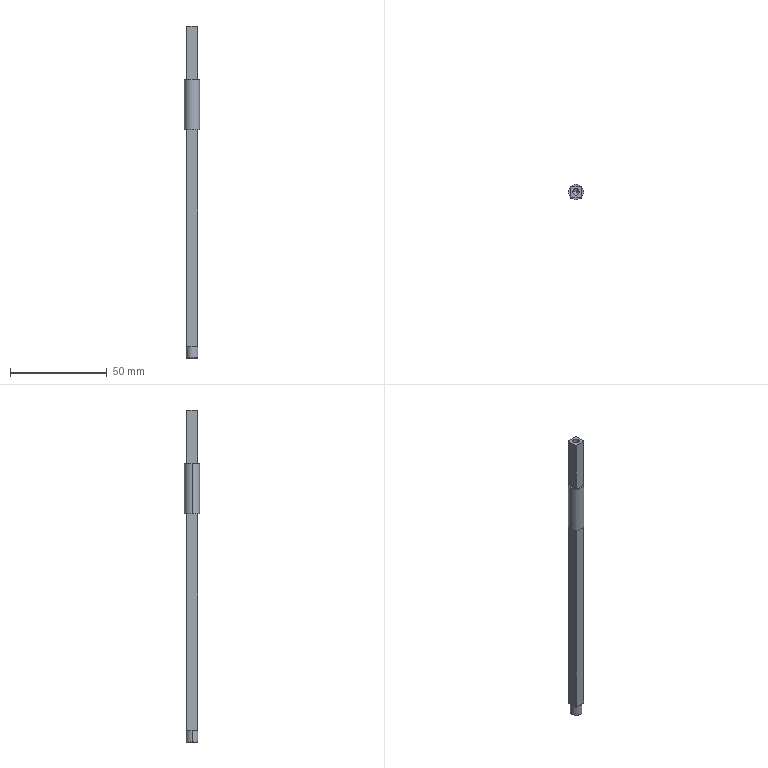Part | NX | features BREP 1 | 1 solid | 36 faces | box 8 x 8 x 172 mm | volume 6270 mm3 | plane 22 | cylinder 8 | cone 6 | commonest cylinder face diameters 3.3 x4 6 x2 8 x2
STEP:
#1=CARTESIAN_POINT('',(-3.,0.,-88.85));
#2=VERTEX_POINT('',#1);
#3=CARTESIAN_POINT('',(-2.85,0.,-89.));
#4=VERTEX_POINT('',#3);
#5=CARTESIAN_POINT('',(-3.,0.,-88.85));
#6=DIRECTION('',(-0.7071,0.,0.7071));
#7=VECTOR('',#6,1000.);
#8=LINE('',#5,#7);
#9=EDGE_CURVE('',#2,#4,#8,.F.);
#10=ORIENTED_EDGE('',*,*,#9,.T.);
#11=CARTESIAN_POINT('',(2.85,0.,-89.));
#12=VERTEX_POINT('',#11);
#13=CARTESIAN_POINT('',(0.,0.,-89.));
#14=DIRECTION('',(0.,0.,-1.));
#15=DIRECTION('',(1.,0.,0.));
#16=AXIS2_PLACEMENT_3D('',#13,#14,#15);
#17=CIRCLE('',#16,2.85);
#18=EDGE_CURVE('',#12,#4,#17,.T.);
#19=ORIENTED_EDGE('',*,*,#18,.F.);
#20=CARTESIAN_POINT('',(3.,0.,-88.85));
#21=VERTEX_POINT('',#20);
#22=CARTESIAN_POINT('',(3.,0.,-88.85));
#23=DIRECTION('',(0.7071,0.,0.7071));
#24=VECTOR('',#23,1000.);
#25=LINE('',#22,#24);
#26=EDGE_CURVE('',#21,#12,#25,.F.);
#27=ORIENTED_EDGE('',*,*,#26,.F.);
#28=CARTESIAN_POINT('',(0.,0.,-88.85));
#29=DIRECTION('',(0.,0.,1.));
#30=DIRECTION('',(1.,0.,0.));
#31=AXIS2_PLACEMENT_3D('',#28,#29,#30);
#32=CIRCLE('',#31,3.);
#33=EDGE_CURVE('',#2,#21,#32,.T.);
#34=ORIENTED_EDGE('',*,*,#33,.F.);
#35=EDGE_LOOP('',(#10,#19,#27,#34));
#36=FACE_BOUND('',#35,.T.);
#37=CARTESIAN_POINT('',(0.,0.,-88.85));
#38=DIRECTION('',(0.,0.,1.));
#39=DIRECTION('',(1.,0.,0.));
#40=AXIS2_PLACEMENT_3D('',#37,#38,#39);
#41=CONICAL_SURFACE('',#40,3.,0.7854);
#42=ADVANCED_FACE('',(#36),#41,.T.);
#43=CARTESIAN_POINT('',(1.65,0.,-76.9));
#44=VERTEX_POINT('',#43);
#45=CARTESIAN_POINT('',(1.65,0.,-89.));
#46=VERTEX_POINT('',#45);
#47=CARTESIAN_POINT('',(1.65,0.,-89.));
#48=DIRECTION('',(0.,0.,-1.));
#49=VECTOR('',#48,1000.);
#50=LINE('',#47,#49);
#51=EDGE_CURVE('',#44,#46,#50,.T.);
#52=ORIENTED_EDGE('',*,*,#51,.F.);
#53=CARTESIAN_POINT('',(-1.65,0.,-76.9));
#54=VERTEX_POINT('',#53);
#55=CARTESIAN_POINT('',(0.,0.,-76.9));
#56=DIRECTION('',(0.,0.,-1.));
#57=DIRECTION('',(-1.,0.,0.));
#58=AXIS2_PLACEMENT_3D('',#55,#56,#57);
#59=CIRCLE('',#58,1.65);
#60=EDGE_CURVE('',#54,#44,#59,.T.);
#61=ORIENTED_EDGE('',*,*,#60,.F.);
#62=CARTESIAN_POINT('',(-1.65,0.,-89.));
#63=VERTEX_POINT('',#62);
#64=CARTESIAN_POINT('',(-1.65,0.,-89.));
#65=DIRECTION('',(0.,0.,-1.));
#66=VECTOR('',#65,1000.);
#67=LINE('',#64,#66);
#68=EDGE_CURVE('',#54,#63,#67,.T.);
#69=ORIENTED_EDGE('',*,*,#68,.T.);
#70=CARTESIAN_POINT('',(0.,0.,-89.));
#71=DIRECTION('',(0.,0.,-1.));
#72=DIRECTION('',(-1.,0.,0.));
#73=AXIS2_PLACEMENT_3D('',#70,#71,#72);
#74=CIRCLE('',#73,1.65);
#75=EDGE_CURVE('',#63,#46,#74,.T.);
#76=ORIENTED_EDGE('',*,*,#75,.T.);
#77=EDGE_LOOP('',(#52,#61,#69,#76));
#78=FACE_BOUND('',#77,.T.);
#79=CARTESIAN_POINT('',(0.,0.,-89.));
#80=DIRECTION('',(0.,0.,-1.));
#81=DIRECTION('',(-1.,0.,0.));
#82=AXIS2_PLACEMENT_3D('',#79,#80,#81);
#83=CYLINDRICAL_SURFACE('',#82,1.65);
#84=ADVANCED_FACE('',(#78),#83,.F.);
#85=CARTESIAN_POINT('',(0.,0.,-75.909));
#86=VERTEX_POINT('',#85);
#87=CARTESIAN_POINT('',(1.65,0.,-76.9));
#88=DIRECTION('',(0.8572,0.,-0.515));
#89=VECTOR('',#88,1000.);
#90=LINE('',#87,#89);
#91=EDGE_CURVE('',#44,#86,#90,.F.);
#92=ORIENTED_EDGE('',*,*,#91,.T.);
#93=CARTESIAN_POINT('',(-1.65,0.,-76.9));
#94=DIRECTION('',(-0.8572,0.,-0.515));
#95=VECTOR('',#94,1000.);
#96=LINE('',#93,#95);
#97=EDGE_CURVE('',#54,#86,#96,.F.);
#98=ORIENTED_EDGE('',*,*,#97,.F.);
#99=ORIENTED_EDGE('',*,*,#60,.T.);
#100=EDGE_LOOP('',(#92,#98,#99));
#101=FACE_BOUND('',#100,.T.);
#102=CARTESIAN_POINT('',(0.,0.,-76.9));
#103=DIRECTION('',(0.,0.,-1.));
#104=DIRECTION('',(-1.,0.,0.));
#105=AXIS2_PLACEMENT_3D('',#102,#103,#104);
#106=CONICAL_SURFACE('',#105,1.65,1.03);
#107=ADVANCED_FACE('',(#101),#106,.F.);
#108=CARTESIAN_POINT('',(-1.65,0.,83.));
#109=VERTEX_POINT('',#108);
#110=CARTESIAN_POINT('',(-1.65,0.,70.9));
#111=VERTEX_POINT('',#110);
#112=CARTESIAN_POINT('',(-1.65,0.,83.));
#113=DIRECTION('',(0.,0.,1.));
#114=VECTOR('',#113,1000.);
#115=LINE('',#112,#114);
#116=EDGE_CURVE('',#109,#111,#115,.F.);
#117=ORIENTED_EDGE('',*,*,#116,.T.);
#118=CARTESIAN_POINT('',(1.65,0.,70.9));
#119=VERTEX_POINT('',#118);
#120=CARTESIAN_POINT('',(0.,0.,70.9));
#121=DIRECTION('',(0.,0.,1.));
#122=DIRECTION('',(1.,0.,0.));
#123=AXIS2_PLACEMENT_3D('',#120,#121,#122);
#124=CIRCLE('',#123,1.65);
#125=EDGE_CURVE('',#119,#111,#124,.T.);
#126=ORIENTED_EDGE('',*,*,#125,.F.);
#127=CARTESIAN_POINT('',(1.65,0.,83.));
#128=VERTEX_POINT('',#127);
#129=CARTESIAN_POINT('',(1.65,0.,83.));
#130=DIRECTION('',(0.,0.,1.));
#131=VECTOR('',#130,1000.);
#132=LINE('',#129,#131);
#133=EDGE_CURVE('',#128,#119,#132,.F.);
#134=ORIENTED_EDGE('',*,*,#133,.F.);
#135=CARTESIAN_POINT('',(0.,0.,83.));
#136=DIRECTION('',(0.,0.,1.));
#137=DIRECTION('',(1.,0.,0.));
#138=AXIS2_PLACEMENT_3D('',#135,#136,#137);
#139=CIRCLE('',#138,1.65);
#140=EDGE_CURVE('',#128,#109,#139,.T.);
#141=ORIENTED_EDGE('',*,*,#140,.T.);
#142=EDGE_LOOP('',(#117,#126,#134,#141));
#143=FACE_BOUND('',#142,.T.);
#144=CARTESIAN_POINT('',(0.,0.,83.));
#145=DIRECTION('',(0.,0.,1.));
#146=DIRECTION('',(1.,0.,0.));
#147=AXIS2_PLACEMENT_3D('',#144,#145,#146);
#148=CYLINDRICAL_SURFACE('',#147,1.65);
#149=ADVANCED_FACE('',(#143),#148,.F.);
#150=CARTESIAN_POINT('',(0.,0.,69.909));
#151=VERTEX_POINT('',#150);
#152=CARTESIAN_POINT('',(-1.65,0.,70.9));
#153=DIRECTION('',(-0.8572,0.,0.515));
#154=VECTOR('',#153,1000.);
#155=LINE('',#152,#154);
#156=EDGE_CURVE('',#151,#111,#155,.T.);
#157=ORIENTED_EDGE('',*,*,#156,.F.);
#158=CARTESIAN_POINT('',(1.65,0.,70.9));
#159=DIRECTION('',(0.8572,0.,0.515));
#160=VECTOR('',#159,1000.);
#161=LINE('',#158,#160);
#162=EDGE_CURVE('',#151,#119,#161,.T.);
#163=ORIENTED_EDGE('',*,*,#162,.T.);
#164=ORIENTED_EDGE('',*,*,#125,.T.);
#165=EDGE_LOOP('',(#157,#163,#164));
#166=FACE_BOUND('',#165,.T.);
#167=CARTESIAN_POINT('',(0.,0.,70.9));
#168=DIRECTION('',(0.,0.,1.));
#169=DIRECTION('',(1.,0.,0.));
#170=AXIS2_PLACEMENT_3D('',#167,#168,#169);
#171=CONICAL_SURFACE('',#170,1.65,1.03);
#172=ADVANCED_FACE('',(#166),#171,.F.);
#173=CARTESIAN_POINT('',(-2.646,-3.,55.25));
#174=VERTEX_POINT('',#173);
#175=CARTESIAN_POINT('',(2.646,-3.,55.25));
#176=VERTEX_POINT('',#175);
#177=CARTESIAN_POINT('',(-2.646,-3.,55.25));
#178=DIRECTION('',(1.,0.,0.));
#179=VECTOR('',#178,1000.);
#180=LINE('',#177,#179);
#181=EDGE_CURVE('',#174,#176,#180,.T.);
#182=ORIENTED_EDGE('',*,*,#181,.F.);
#183=CARTESIAN_POINT('',(0.,0.,55.25));
#184=DIRECTION('',(0.,0.,1.));
#185=DIRECTION('',(1.,0.,0.));
#186=AXIS2_PLACEMENT_3D('',#183,#184,#185);
#187=CIRCLE('',#186,4.);
#188=EDGE_CURVE('',#174,#176,#187,.T.);
#189=ORIENTED_EDGE('',*,*,#188,.T.);
#190=EDGE_LOOP('',(#182,#189));
#191=FACE_BOUND('',#190,.T.);
#192=CARTESIAN_POINT('',(0.,0.,55.25));
#193=DIRECTION('',(0.,0.,1.));
#194=DIRECTION('',(1.,0.,0.));
#195=AXIS2_PLACEMENT_3D('',#192,#193,#194);
#196=PLANE('',#195);
#197=ADVANCED_FACE('',(#191),#196,.T.);
#198=CARTESIAN_POINT('',(-2.646,-3.,29.25));
#199=VERTEX_POINT('',#198);
#200=CARTESIAN_POINT('',(2.646,-3.,29.25));
#201=VERTEX_POINT('',#200);
#202=CARTESIAN_POINT('',(0.,0.,29.25));
#203=DIRECTION('',(0.,0.,1.));
#204=DIRECTION('',(1.,0.,0.));
#205=AXIS2_PLACEMENT_3D('',#202,#203,#204);
#206=CIRCLE('',#205,4.);
#207=EDGE_CURVE('',#199,#201,#206,.T.);
#208=ORIENTED_EDGE('',*,*,#207,.F.);
#209=CARTESIAN_POINT('',(-2.646,-3.,29.25));
#210=DIRECTION('',(1.,0.,0.));
#211=VECTOR('',#210,1000.);
#212=LINE('',#209,#211);
#213=EDGE_CURVE('',#199,#201,#212,.T.);
#214=ORIENTED_EDGE('',*,*,#213,.T.);
#215=EDGE_LOOP('',(#208,#214));
#216=FACE_BOUND('',#215,.T.);
#217=CARTESIAN_POINT('',(0.,0.,29.25));
#218=DIRECTION('',(0.,0.,1.));
#219=DIRECTION('',(1.,0.,0.));
#220=AXIS2_PLACEMENT_3D('',#217,#218,#219);
#221=PLANE('',#220);
#222=ADVANCED_FACE('',(#216),#221,.F.);
#223=CARTESIAN_POINT('',(3.,-2.646,29.25));
#224=VERTEX_POINT('',#223);
#225=CARTESIAN_POINT('',(4.,0.,29.25));
#226=VERTEX_POINT('',#225);
#227=CARTESIAN_POINT('',(0.,0.,29.25));
#228=DIRECTION('',(0.,0.,1.));
#229=DIRECTION('',(1.,0.,0.));
#230=AXIS2_PLACEMENT_3D('',#227,#228,#229);
#231=CIRCLE('',#230,4.);
#232=EDGE_CURVE('',#224,#226,#231,.T.);
#233=ORIENTED_EDGE('',*,*,#232,.F.);
#234=CARTESIAN_POINT('',(3.,2.646,29.25));
#235=VERTEX_POINT('',#234);
#236=CARTESIAN_POINT('',(3.,-2.646,29.25));
#237=DIRECTION('',(0.,1.,0.));
#238=VECTOR('',#237,1000.);
#239=LINE('',#236,#238);
#240=EDGE_CURVE('',#224,#235,#239,.T.);
#241=ORIENTED_EDGE('',*,*,#240,.T.);
#242=CARTESIAN_POINT('',(0.,0.,29.25));
#243=DIRECTION('',(0.,0.,1.));
#244=DIRECTION('',(1.,0.,0.));
#245=AXIS2_PLACEMENT_3D('',#242,#243,#244);
#246=CIRCLE('',#245,4.);
#247=EDGE_CURVE('',#226,#235,#246,.T.);
#248=ORIENTED_EDGE('',*,*,#247,.F.);
#249=EDGE_LOOP('',(#233,#241,#248));
#250=FACE_BOUND('',#249,.T.);
#251=CARTESIAN_POINT('',(0.,0.,29.25));
#252=DIRECTION('',(0.,0.,1.));
#253=DIRECTION('',(1.,0.,0.));
#254=AXIS2_PLACEMENT_3D('',#251,#252,#253);
#255=PLANE('',#254);
#256=ADVANCED_FACE('',(#250),#255,.F.);
#257=CARTESIAN_POINT('',(3.,-2.646,55.25));
#258=VERTEX_POINT('',#257);
#259=CARTESIAN_POINT('',(3.,2.646,55.25));
#260=VERTEX_POINT('',#259);
#261=CARTESIAN_POINT('',(3.,-2.646,55.25));
#262=DIRECTION('',(0.,1.,0.));
#263=VECTOR('',#262,1000.);
#264=LINE('',#261,#263);
#265=EDGE_CURVE('',#258,#260,#264,.T.);
#266=ORIENTED_EDGE('',*,*,#265,.F.);
#267=CARTESIAN_POINT('',(4.,0.,55.25));
#268=VERTEX_POINT('',#267);
#269=CARTESIAN_POINT('',(0.,0.,55.25));
#270=DIRECTION('',(0.,0.,1.));
#271=DIRECTION('',(1.,0.,0.));
#272=AXIS2_PLACEMENT_3D('',#269,#270,#271);
#273=CIRCLE('',#272,4.);
#274=EDGE_CURVE('',#258,#268,#273,.T.);
#275=ORIENTED_EDGE('',*,*,#274,.T.);
#276=CARTESIAN_POINT('',(0.,0.,55.25));
#277=DIRECTION('',(0.,0.,1.));
#278=DIRECTION('',(1.,0.,0.));
#279=AXIS2_PLACEMENT_3D('',#276,#277,#278);
#280=CIRCLE('',#279,4.);
#281=EDGE_CURVE('',#268,#260,#280,.T.);
#282=ORIENTED_EDGE('',*,*,#281,.T.);
#283=EDGE_LOOP('',(#266,#275,#282));
#284=FACE_BOUND('',#283,.T.);
#285=CARTESIAN_POINT('',(0.,0.,55.25));
#286=DIRECTION('',(0.,0.,1.));
#287=DIRECTION('',(1.,0.,0.));
#288=AXIS2_PLACEMENT_3D('',#285,#286,#287);
#289=PLANE('',#288);
#290=ADVANCED_FACE('',(#284),#289,.T.);
#291=CARTESIAN_POINT('',(2.646,3.,29.25));
#292=VERTEX_POINT('',#291);
#293=CARTESIAN_POINT('',(-2.646,3.,29.25));
#294=VERTEX_POINT('',#293);
#295=CARTESIAN_POINT('',(0.,0.,29.25));
#296=DIRECTION('',(0.,0.,1.));
#297=DIRECTION('',(1.,0.,0.));
#298=AXIS2_PLACEMENT_3D('',#295,#296,#297);
#299=CIRCLE('',#298,4.);
#300=EDGE_CURVE('',#292,#294,#299,.T.);
#301=ORIENTED_EDGE('',*,*,#300,.F.);
#302=CARTESIAN_POINT('',(-2.646,3.,29.25));
#303=DIRECTION('',(-1.,0.,0.));
#304=VECTOR('',#303,1000.);
#305=LINE('',#302,#304);
#306=EDGE_CURVE('',#292,#294,#305,.T.);
#307=ORIENTED_EDGE('',*,*,#306,.T.);
#308=EDGE_LOOP('',(#301,#307));
#309=FACE_BOUND('',#308,.T.);
#310=CARTESIAN_POINT('',(0.,0.,29.25));
#311=DIRECTION('',(0.,0.,1.));
#312=DIRECTION('',(1.,0.,0.));
#313=AXIS2_PLACEMENT_3D('',#310,#311,#312);
#314=PLANE('',#313);
#315=ADVANCED_FACE('',(#309),#314,.F.);
#316=CARTESIAN_POINT('',(2.646,3.,55.25));
#317=VERTEX_POINT('',#316);
#318=CARTESIAN_POINT('',(-2.646,3.,55.25));
#319=VERTEX_POINT('',#318);
#320=CARTESIAN_POINT('',(-2.646,3.,55.25));
#321=DIRECTION('',(-1.,0.,0.));
#322=VECTOR('',#321,1000.);
#323=LINE('',#320,#322);
#324=EDGE_CURVE('',#317,#319,#323,.T.);
#325=ORIENTED_EDGE('',*,*,#324,.F.);
#326=CARTESIAN_POINT('',(0.,0.,55.25));
#327=DIRECTION('',(0.,0.,1.));
#328=DIRECTION('',(1.,0.,0.));
#329=AXIS2_PLACEMENT_3D('',#326,#327,#328);
#330=CIRCLE('',#329,4.);
#331=EDGE_CURVE('',#317,#319,#330,.T.);
#332=ORIENTED_EDGE('',*,*,#331,.T.);
#333=EDGE_LOOP('',(#325,#332));
#334=FACE_BOUND('',#333,.T.);
#335=CARTESIAN_POINT('',(0.,0.,55.25));
#336=DIRECTION('',(0.,0.,1.));
#337=DIRECTION('',(1.,0.,0.));
#338=AXIS2_PLACEMENT_3D('',#335,#336,#337);
#339=PLANE('',#338);
#340=ADVANCED_FACE('',(#334),#339,.T.);
#341=CARTESIAN_POINT('',(-3.,2.646,29.25));
#342=VERTEX_POINT('',#341);
#343=CARTESIAN_POINT('',(-4.,0.,29.25));
#344=VERTEX_POINT('',#343);
#345=CARTESIAN_POINT('',(0.,0.,29.25));
#346=DIRECTION('',(0.,0.,1.));
#347=DIRECTION('',(1.,0.,0.));
#348=AXIS2_PLACEMENT_3D('',#345,#346,#347);
#349=CIRCLE('',#348,4.);
#350=EDGE_CURVE('',#342,#344,#349,.T.);
#351=ORIENTED_EDGE('',*,*,#350,.F.);
#352=CARTESIAN_POINT('',(-3.,-2.646,29.25));
#353=VERTEX_POINT('',#352);
#354=CARTESIAN_POINT('',(-3.,-2.646,29.25));
#355=DIRECTION('',(0.,-1.,0.));
#356=VECTOR('',#355,1000.);
#357=LINE('',#354,#356);
#358=EDGE_CURVE('',#342,#353,#357,.T.);
#359=ORIENTED_EDGE('',*,*,#358,.T.);
#360=CARTESIAN_POINT('',(0.,0.,29.25));
#361=DIRECTION('',(0.,0.,1.));
#362=DIRECTION('',(1.,0.,0.));
#363=AXIS2_PLACEMENT_3D('',#360,#361,#362);
#364=CIRCLE('',#363,4.);
#365=EDGE_CURVE('',#344,#353,#364,.T.);
#366=ORIENTED_EDGE('',*,*,#365,.F.);
#367=EDGE_LOOP('',(#351,#359,#366));
#368=FACE_BOUND('',#367,.T.);
#369=CARTESIAN_POINT('',(0.,0.,29.25));
#370=DIRECTION('',(0.,0.,1.));
#371=DIRECTION('',(1.,0.,0.));
#372=AXIS2_PLACEMENT_3D('',#369,#370,#371);
#373=PLANE('',#372);
#374=ADVANCED_FACE('',(#368),#373,.F.);
#375=CARTESIAN_POINT('',(-3.,2.646,55.25));
#376=VERTEX_POINT('',#375);
#377=CARTESIAN_POINT('',(-3.,-2.646,55.25));
#378=VERTEX_POINT('',#377);
#379=CARTESIAN_POINT('',(-3.,-2.646,55.25));
#380=DIRECTION('',(0.,-1.,0.));
#381=VECTOR('',#380,1000.);
#382=LINE('',#379,#381);
#383=EDGE_CURVE('',#376,#378,#382,.T.);
#384=ORIENTED_EDGE('',*,*,#383,.F.);
#385=CARTESIAN_POINT('',(-4.,0.,55.25));
#386=VERTEX_POINT('',#385);
#387=CARTESIAN_POINT('',(0.,0.,55.25));
#388=DIRECTION('',(0.,0.,1.));
#389=DIRECTION('',(1.,0.,0.));
#390=AXIS2_PLACEMENT_3D('',#387,#388,#389);
#391=CIRCLE('',#390,4.);
#392=EDGE_CURVE('',#376,#386,#391,.T.);
#393=ORIENTED_EDGE('',*,*,#392,.T.);
#394=CARTESIAN_POINT('',(0.,0.,55.25));
#395=DIRECTION('',(0.,0.,1.));
#396=DIRECTION('',(1.,0.,0.));
#397=AXIS2_PLACEMENT_3D('',#394,#395,#396);
#398=CIRCLE('',#397,4.);
#399=EDGE_CURVE('',#386,#378,#398,.T.);
#400=ORIENTED_EDGE('',*,*,#399,.T.);
#401=EDGE_LOOP('',(#384,#393,#400));
#402=FACE_BOUND('',#401,.T.);
#403=CARTESIAN_POINT('',(0.,0.,55.25));
#404=DIRECTION('',(0.,0.,1.));
#405=DIRECTION('',(1.,0.,0.));
#406=AXIS2_PLACEMENT_3D('',#403,#404,#405);
#407=PLANE('',#406);
#408=ADVANCED_FACE('',(#402),#407,.T.);
#409=ORIENTED_EDGE('',*,*,#75,.F.);
#410=CARTESIAN_POINT('',(0.,0.,-89.));
#411=DIRECTION('',(0.,0.,-1.));
#412=DIRECTION('',(-1.,0.,0.));
#413=AXIS2_PLACEMENT_3D('',#410,#411,#412);
#414=CIRCLE('',#413,1.65);
#415=EDGE_CURVE('',#46,#63,#414,.T.);
#416=ORIENTED_EDGE('',*,*,#415,.F.);
#417=EDGE_LOOP('',(#409,#416));
#418=FACE_BOUND('',#417,.T.);
#419=ORIENTED_EDGE('',*,*,#18,.T.);
#420=CARTESIAN_POINT('',(0.,0.,-89.));
#421=DIRECTION('',(0.,0.,-1.));
#422=DIRECTION('',(1.,0.,0.));
#423=AXIS2_PLACEMENT_3D('',#420,#421,#422);
#424=CIRCLE('',#423,2.85);
#425=EDGE_CURVE('',#4,#12,#424,.T.);
#426=ORIENTED_EDGE('',*,*,#425,.T.);
#427=EDGE_LOOP('',(#419,#426));
#428=FACE_BOUND('',#427,.T.);
#429=CARTESIAN_POINT('',(-3.,0.,-89.));
#430=DIRECTION('',(0.,0.,1.));
#431=DIRECTION('',(1.,0.,0.));
#432=AXIS2_PLACEMENT_3D('',#429,#430,#431);
#433=PLANE('',#432);
#434=ADVANCED_FACE('',(#418,#428),#433,.F.);
#435=CARTESIAN_POINT('',(-3.,0.,-83.));
#436=VERTEX_POINT('',#435);
#437=CARTESIAN_POINT('',(-3.,0.,0.));
#438=DIRECTION('',(0.,0.,1.));
#439=VECTOR('',#438,1000.);
#440=LINE('',#437,#439);
#441=EDGE_CURVE('',#436,#2,#440,.F.);
#442=ORIENTED_EDGE('',*,*,#441,.T.);
#443=ORIENTED_EDGE('',*,*,#33,.T.);
#444=CARTESIAN_POINT('',(3.,0.,-83.));
#445=VERTEX_POINT('',#444);
#446=CARTESIAN_POINT('',(3.,0.,0.));
#447=DIRECTION('',(0.,0.,1.));
#448=VECTOR('',#447,1000.);
#449=LINE('',#446,#448);
#450=EDGE_CURVE('',#445,#21,#449,.F.);
#451=ORIENTED_EDGE('',*,*,#450,.F.);
#452=CARTESIAN_POINT('',(0.,-3.,-83.));
#453=VERTEX_POINT('',#452);
#454=CARTESIAN_POINT('',(0.,0.,-83.));
#455=DIRECTION('',(0.,0.,1.));
#456=DIRECTION('',(1.,0.,0.));
#457=AXIS2_PLACEMENT_3D('',#454,#455,#456);
#458=CIRCLE('',#457,3.);
#459=EDGE_CURVE('',#453,#445,#458,.T.);
#460=ORIENTED_EDGE('',*,*,#459,.F.);
#461=CARTESIAN_POINT('',(0.,0.,-83.));
#462=DIRECTION('',(0.,0.,1.));
#463=DIRECTION('',(1.,0.,0.));
#464=AXIS2_PLACEMENT_3D('',#461,#462,#463);
#465=CIRCLE('',#464,3.);
#466=EDGE_CURVE('',#436,#453,#465,.T.);
#467=ORIENTED_EDGE('',*,*,#466,.F.);
#468=EDGE_LOOP('',(#442,#443,#451,#460,#467));
#469=FACE_BOUND('',#468,.T.);
#470=CARTESIAN_POINT('',(0.,0.,0.));
#471=DIRECTION('',(0.,0.,1.));
#472=DIRECTION('',(1.,0.,0.));
#473=AXIS2_PLACEMENT_3D('',#470,#471,#472);
#474=CYLINDRICAL_SURFACE('',#473,3.);
#475=ADVANCED_FACE('',(#469),#474,.T.);
#476=CARTESIAN_POINT('',(2.646,-3.,-83.));
#477=VERTEX_POINT('',#476);
#478=CARTESIAN_POINT('',(-2.646,-3.,-83.));
#479=DIRECTION('',(1.,0.,0.));
#480=VECTOR('',#479,1000.);
#481=LINE('',#478,#480);
#482=EDGE_CURVE('',#453,#477,#481,.T.);
#483=ORIENTED_EDGE('',*,*,#482,.F.);
#484=ORIENTED_EDGE('',*,*,#459,.T.);
#485=CARTESIAN_POINT('',(3.,-2.646,-83.));
#486=VERTEX_POINT('',#485);
#487=CARTESIAN_POINT('',(3.,-2.646,-83.));
#488=DIRECTION('',(0.,1.,0.));
#489=VECTOR('',#488,1000.);
#490=LINE('',#487,#489);
#491=EDGE_CURVE('',#486,#445,#490,.T.);
#492=ORIENTED_EDGE('',*,*,#491,.F.);
#493=CARTESIAN_POINT('',(0.,0.,-83.));
#494=DIRECTION('',(0.,0.,1.));
#495=DIRECTION('',(1.,0.,0.));
#496=AXIS2_PLACEMENT_3D('',#493,#494,#495);
#497=CIRCLE('',#496,4.);
#498=EDGE_CURVE('',#477,#486,#497,.T.);
#499=ORIENTED_EDGE('',*,*,#498,.F.);
#500=EDGE_LOOP('',(#483,#484,#492,#499));
#501=FACE_BOUND('',#500,.T.);
#502=CARTESIAN_POINT('',(0.,0.,-83.));
#503=DIRECTION('',(0.,0.,1.));
#504=DIRECTION('',(1.,0.,0.));
#505=AXIS2_PLACEMENT_3D('',#502,#503,#504);
#506=PLANE('',#505);
#507=ADVANCED_FACE('',(#501),#506,.F.);
#508=CARTESIAN_POINT('',(-3.,-2.646,83.));
#509=VERTEX_POINT('',#508);
#510=CARTESIAN_POINT('',(-2.646,-3.,83.));
#511=VERTEX_POINT('',#510);
#512=CARTESIAN_POINT('',(0.,0.,83.));
#513=DIRECTION('',(0.,0.,1.));
#514=DIRECTION('',(1.,0.,0.));
#515=AXIS2_PLACEMENT_3D('',#512,#513,#514);
#516=CIRCLE('',#515,4.);
#517=EDGE_CURVE('',#509,#511,#516,.T.);
#518=ORIENTED_EDGE('',*,*,#517,.T.);
#519=CARTESIAN_POINT('',(2.646,-3.,83.));
#520=VERTEX_POINT('',#519);
#521=CARTESIAN_POINT('',(-2.646,-3.,83.));
#522=DIRECTION('',(1.,0.,0.));
#523=VECTOR('',#522,1000.);
#524=LINE('',#521,#523);
#525=EDGE_CURVE('',#511,#520,#524,.T.);
#526=ORIENTED_EDGE('',*,*,#525,.T.);
#527=CARTESIAN_POINT('',(3.,-2.646,83.));
#528=VERTEX_POINT('',#527);
#529=CARTESIAN_POINT('',(0.,0.,83.));
#530=DIRECTION('',(0.,0.,1.));
#531=DIRECTION('',(1.,0.,0.));
#532=AXIS2_PLACEMENT_3D('',#529,#530,#531);
#533=CIRCLE('',#532,4.);
#534=EDGE_CURVE('',#520,#528,#533,.T.);
#535=ORIENTED_EDGE('',*,*,#534,.T.);
#536=CARTESIAN_POINT('',(3.,2.646,83.));
#537=VERTEX_POINT('',#536);
#538=CARTESIAN_POINT('',(3.,-2.646,83.));
#539=DIRECTION('',(0.,1.,0.));
#540=VECTOR('',#539,1000.);
#541=LINE('',#538,#540);
#542=EDGE_CURVE('',#528,#537,#541,.T.);
#543=ORIENTED_EDGE('',*,*,#542,.T.);
#544=CARTESIAN_POINT('',(2.646,3.,83.));
#545=VERTEX_POINT('',#544);
#546=CARTESIAN_POINT('',(0.,0.,83.));
#547=DIRECTION('',(0.,0.,1.));
#548=DIRECTION('',(1.,0.,0.));
#549=AXIS2_PLACEMENT_3D('',#546,#547,#548);
#550=CIRCLE('',#549,4.);
#551=EDGE_CURVE('',#537,#545,#550,.T.);
#552=ORIENTED_EDGE('',*,*,#551,.T.);
#553=CARTESIAN_POINT('',(-2.646,3.,83.));
#554=VERTEX_POINT('',#553);
#555=CARTESIAN_POINT('',(-2.646,3.,83.));
#556=DIRECTION('',(-1.,0.,0.));
#557=VECTOR('',#556,1000.);
#558=LINE('',#555,#557);
#559=EDGE_CURVE('',#545,#554,#558,.T.);
#560=ORIENTED_EDGE('',*,*,#559,.T.);
#561=CARTESIAN_POINT('',(-3.,2.646,83.));
#562=VERTEX_POINT('',#561);
#563=CARTESIAN_POINT('',(0.,0.,83.));
#564=DIRECTION('',(0.,0.,1.));
#565=DIRECTION('',(1.,0.,0.));
#566=AXIS2_PLACEMENT_3D('',#563,#564,#565);
#567=CIRCLE('',#566,4.);
#568=EDGE_CURVE('',#554,#562,#567,.T.);
#569=ORIENTED_EDGE('',*,*,#568,.T.);
#570=CARTESIAN_POINT('',(-3.,-2.646,83.));
#571=DIRECTION('',(0.,-1.,0.));
#572=VECTOR('',#571,1000.);
#573=LINE('',#570,#572);
#574=EDGE_CURVE('',#562,#509,#573,.T.);
#575=ORIENTED_EDGE('',*,*,#574,.T.);
#576=EDGE_LOOP('',(#518,#526,#535,#543,#552,#560,#569,#575));
#577=FACE_BOUND('',#576,.T.);
#578=ORIENTED_EDGE('',*,*,#140,.F.);
#579=CARTESIAN_POINT('',(0.,0.,83.));
#580=DIRECTION('',(0.,0.,1.));
#581=DIRECTION('',(1.,0.,0.));
#582=AXIS2_PLACEMENT_3D('',#579,#580,#581);
#583=CIRCLE('',#582,1.65);
#584=EDGE_CURVE('',#109,#128,#583,.T.);
#585=ORIENTED_EDGE('',*,*,#584,.F.);
#586=EDGE_LOOP('',(#578,#585));
#587=FACE_BOUND('',#586,.T.);
#588=CARTESIAN_POINT('',(0.,0.,83.));
#589=DIRECTION('',(0.,0.,1.));
#590=DIRECTION('',(1.,0.,0.));
#591=AXIS2_PLACEMENT_3D('',#588,#589,#590);
#592=PLANE('',#591);
#593=ADVANCED_FACE('',(#577,#587),#592,.T.);
#594=CARTESIAN_POINT('',(-3.,2.646,83.));
#595=DIRECTION('',(0.,0.,-1.));
#596=VECTOR('',#595,1000.);
#597=LINE('',#594,#596);
#598=EDGE_CURVE('',#562,#376,#597,.T.);
#599=ORIENTED_EDGE('',*,*,#598,.T.);
#600=ORIENTED_EDGE('',*,*,#383,.T.);
#601=CARTESIAN_POINT('',(-3.,-2.646,83.));
#602=DIRECTION('',(0.,0.,-1.));
#603=VECTOR('',#602,1000.);
#604=LINE('',#601,#603);
#605=EDGE_CURVE('',#509,#378,#604,.T.);
#606=ORIENTED_EDGE('',*,*,#605,.F.);
#607=ORIENTED_EDGE('',*,*,#574,.F.);
#608=EDGE_LOOP('',(#599,#600,#606,#607));
#609=FACE_BOUND('',#608,.T.);
#610=CARTESIAN_POINT('',(-3.,-2.646,83.));
#611=DIRECTION('',(1.,0.,0.));
#612=DIRECTION('',(0.,0.,-1.));
#613=AXIS2_PLACEMENT_3D('',#610,#611,#612);
#614=PLANE('',#613);
#615=ADVANCED_FACE('',(#609),#614,.F.);
#616=CARTESIAN_POINT('',(4.,0.,83.));
#617=DIRECTION('',(0.,0.,-1.));
#618=VECTOR('',#617,1000.);
#619=LINE('',#616,#618);
#620=EDGE_CURVE('',#268,#226,#619,.T.);
#621=ORIENTED_EDGE('',*,*,#620,.F.);
#622=ORIENTED_EDGE('',*,*,#274,.F.);
#623=CARTESIAN_POINT('',(3.,-2.646,83.));
#624=DIRECTION('',(0.,0.,-1.));
#625=VECTOR('',#624,1000.);
#626=LINE('',#623,#625);
#627=EDGE_CURVE('',#528,#258,#626,.T.);
#628=ORIENTED_EDGE('',*,*,#627,.F.);
#629=ORIENTED_EDGE('',*,*,#534,.F.);
#630=CARTESIAN_POINT('',(2.646,-3.,83.));
#631=DIRECTION('',(0.,0.,-1.));
#632=VECTOR('',#631,1000.);
#633=LINE('',#630,#632);
#634=EDGE_CURVE('',#176,#520,#633,.F.);
#635=ORIENTED_EDGE('',*,*,#634,.F.);
#636=ORIENTED_EDGE('',*,*,#188,.F.);
#637=CARTESIAN_POINT('',(-2.646,-3.,83.));
#638=DIRECTION('',(0.,0.,-1.));
#639=VECTOR('',#638,1000.);
#640=LINE('',#637,#639);
#641=EDGE_CURVE('',#174,#511,#640,.F.);
#642=ORIENTED_EDGE('',*,*,#641,.T.);
#643=ORIENTED_EDGE('',*,*,#517,.F.);
#644=ORIENTED_EDGE('',*,*,#605,.T.);
#645=ORIENTED_EDGE('',*,*,#399,.F.);
#646=CARTESIAN_POINT('',(-4.,0.,83.));
#647=DIRECTION('',(0.,0.,-1.));
#648=VECTOR('',#647,1000.);
#649=LINE('',#646,#648);
#650=EDGE_CURVE('',#386,#344,#649,.T.);
#651=ORIENTED_EDGE('',*,*,#650,.T.);
#652=ORIENTED_EDGE('',*,*,#365,.T.);
#653=CARTESIAN_POINT('',(-3.,-2.646,-83.));
#654=VERTEX_POINT('',#653);
#655=CARTESIAN_POINT('',(-3.,-2.646,83.));
#656=DIRECTION('',(0.,0.,-1.));
#657=VECTOR('',#656,1000.);
#658=LINE('',#655,#657);
#659=EDGE_CURVE('',#353,#654,#658,.T.);
#660=ORIENTED_EDGE('',*,*,#659,.T.);
#661=CARTESIAN_POINT('',(-2.646,-3.,-83.));
#662=VERTEX_POINT('',#661);
#663=CARTESIAN_POINT('',(0.,0.,-83.));
#664=DIRECTION('',(0.,0.,1.));
#665=DIRECTION('',(1.,0.,0.));
#666=AXIS2_PLACEMENT_3D('',#663,#664,#665);
#667=CIRCLE('',#666,4.);
#668=EDGE_CURVE('',#654,#662,#667,.T.);
#669=ORIENTED_EDGE('',*,*,#668,.T.);
#670=CARTESIAN_POINT('',(-2.646,-3.,83.));
#671=DIRECTION('',(0.,0.,-1.));
#672=VECTOR('',#671,1000.);
#673=LINE('',#670,#672);
#674=EDGE_CURVE('',#662,#199,#673,.F.);
#675=ORIENTED_EDGE('',*,*,#674,.T.);
#676=ORIENTED_EDGE('',*,*,#207,.T.);
#677=CARTESIAN_POINT('',(2.646,-3.,83.));
#678=DIRECTION('',(0.,0.,-1.));
#679=VECTOR('',#678,1000.);
#680=LINE('',#677,#679);
#681=EDGE_CURVE('',#477,#201,#680,.F.);
#682=ORIENTED_EDGE('',*,*,#681,.F.);
#683=ORIENTED_EDGE('',*,*,#498,.T.);
#684=CARTESIAN_POINT('',(3.,-2.646,83.));
#685=DIRECTION('',(0.,0.,-1.));
#686=VECTOR('',#685,1000.);
#687=LINE('',#684,#686);
#688=EDGE_CURVE('',#224,#486,#687,.T.);
#689=ORIENTED_EDGE('',*,*,#688,.F.);
#690=ORIENTED_EDGE('',*,*,#232,.T.);
#691=EDGE_LOOP('',(#621,#622,#628,#629,#635,#636,#642,#643,#644,#645,#651,#652,#660,#669,#675,#676,#682,#683,#689,#690));
#692=FACE_BOUND('',#691,.T.);
#693=CARTESIAN_POINT('',(0.,0.,83.));
#694=DIRECTION('',(0.,0.,-1.));
#695=DIRECTION('',(-1.,0.,0.));
#696=AXIS2_PLACEMENT_3D('',#693,#694,#695);
#697=CYLINDRICAL_SURFACE('',#696,4.);
#698=ADVANCED_FACE('',(#692),#697,.T.);
#699=CARTESIAN_POINT('',(2.646,3.,83.));
#700=DIRECTION('',(0.,0.,-1.));
#701=VECTOR('',#700,1000.);
#702=LINE('',#699,#701);
#703=EDGE_CURVE('',#317,#545,#702,.F.);
#704=ORIENTED_EDGE('',*,*,#703,.F.);
#705=ORIENTED_EDGE('',*,*,#324,.T.);
#706=CARTESIAN_POINT('',(-2.646,3.,83.));
#707=DIRECTION('',(0.,0.,-1.));
#708=VECTOR('',#707,1000.);
#709=LINE('',#706,#708);
#710=EDGE_CURVE('',#319,#554,#709,.F.);
#711=ORIENTED_EDGE('',*,*,#710,.T.);
#712=ORIENTED_EDGE('',*,*,#559,.F.);
#713=EDGE_LOOP('',(#704,#705,#711,#712));
#714=FACE_BOUND('',#713,.T.);
#715=CARTESIAN_POINT('',(-2.646,3.,83.));
#716=DIRECTION('',(0.,-1.,0.));
#717=DIRECTION('',(0.,0.,-1.));
#718=AXIS2_PLACEMENT_3D('',#715,#716,#717);
#719=PLANE('',#718);
#720=ADVANCED_FACE('',(#714),#719,.F.);
#721=ORIENTED_EDGE('',*,*,#627,.T.);
#722=ORIENTED_EDGE('',*,*,#265,.T.);
#723=CARTESIAN_POINT('',(3.,2.646,83.));
#724=DIRECTION('',(0.,0.,-1.));
#725=VECTOR('',#724,1000.);
#726=LINE('',#723,#725);
#727=EDGE_CURVE('',#537,#260,#726,.T.);
#728=ORIENTED_EDGE('',*,*,#727,.F.);
#729=ORIENTED_EDGE('',*,*,#542,.F.);
#730=EDGE_LOOP('',(#721,#722,#728,#729));
#731=FACE_BOUND('',#730,.T.);
#732=CARTESIAN_POINT('',(3.,-2.646,83.));
#733=DIRECTION('',(-1.,0.,0.));
#734=DIRECTION('',(0.,-1.,0.));
#735=AXIS2_PLACEMENT_3D('',#732,#733,#734);
#736=PLANE('',#735);
#737=ADVANCED_FACE('',(#731),#736,.F.);
#738=ORIENTED_EDGE('',*,*,#641,.F.);
#739=ORIENTED_EDGE('',*,*,#181,.T.);
#740=ORIENTED_EDGE('',*,*,#634,.T.);
#741=ORIENTED_EDGE('',*,*,#525,.F.);
#742=EDGE_LOOP('',(#738,#739,#740,#741));
#743=FACE_BOUND('',#742,.T.);
#744=CARTESIAN_POINT('',(-2.646,-3.,83.));
#745=DIRECTION('',(0.,1.,0.));
#746=DIRECTION('',(0.,0.,1.));
#747=AXIS2_PLACEMENT_3D('',#744,#745,#746);
#748=PLANE('',#747);
#749=ADVANCED_FACE('',(#743),#748,.F.);
#750=CARTESIAN_POINT('',(-3.,-2.646,-83.));
#751=DIRECTION('',(0.,-1.,0.));
#752=VECTOR('',#751,1000.);
#753=LINE('',#750,#752);
#754=EDGE_CURVE('',#436,#654,#753,.T.);
#755=ORIENTED_EDGE('',*,*,#754,.F.);
#756=ORIENTED_EDGE('',*,*,#466,.T.);
#757=CARTESIAN_POINT('',(-2.646,-3.,-83.));
#758=DIRECTION('',(1.,0.,0.));
#759=VECTOR('',#758,1000.);
#760=LINE('',#757,#759);
#761=EDGE_CURVE('',#662,#453,#760,.T.);
#762=ORIENTED_EDGE('',*,*,#761,.F.);
#763=ORIENTED_EDGE('',*,*,#668,.F.);
#764=EDGE_LOOP('',(#755,#756,#762,#763));
#765=FACE_BOUND('',#764,.T.);
#766=CARTESIAN_POINT('',(0.,0.,-83.));
#767=DIRECTION('',(0.,0.,1.));
#768=DIRECTION('',(1.,0.,0.));
#769=AXIS2_PLACEMENT_3D('',#766,#767,#768);
#770=PLANE('',#769);
#771=ADVANCED_FACE('',(#765),#770,.F.);
#772=CARTESIAN_POINT('',(0.,3.,-83.));
#773=VERTEX_POINT('',#772);
#774=CARTESIAN_POINT('',(-2.646,3.,-83.));
#775=VERTEX_POINT('',#774);
#776=CARTESIAN_POINT('',(-2.646,3.,-83.));
#777=DIRECTION('',(-1.,0.,0.));
#778=VECTOR('',#777,1000.);
#779=LINE('',#776,#778);
#780=EDGE_CURVE('',#773,#775,#779,.T.);
#781=ORIENTED_EDGE('',*,*,#780,.F.);
#782=CARTESIAN_POINT('',(0.,0.,-83.));
#783=DIRECTION('',(0.,0.,1.));
#784=DIRECTION('',(1.,0.,0.));
#785=AXIS2_PLACEMENT_3D('',#782,#783,#784);
#786=CIRCLE('',#785,3.);
#787=EDGE_CURVE('',#773,#436,#786,.T.);
#788=ORIENTED_EDGE('',*,*,#787,.T.);
#789=CARTESIAN_POINT('',(-3.,2.646,-83.));
#790=VERTEX_POINT('',#789);
#791=CARTESIAN_POINT('',(-3.,-2.646,-83.));
#792=DIRECTION('',(0.,-1.,0.));
#793=VECTOR('',#792,1000.);
#794=LINE('',#791,#793);
#795=EDGE_CURVE('',#790,#436,#794,.T.);
#796=ORIENTED_EDGE('',*,*,#795,.F.);
#797=CARTESIAN_POINT('',(0.,0.,-83.));
#798=DIRECTION('',(0.,0.,1.));
#799=DIRECTION('',(1.,0.,0.));
#800=AXIS2_PLACEMENT_3D('',#797,#798,#799);
#801=CIRCLE('',#800,4.);
#802=EDGE_CURVE('',#775,#790,#801,.T.);
#803=ORIENTED_EDGE('',*,*,#802,.F.);
#804=EDGE_LOOP('',(#781,#788,#796,#803));
#805=FACE_BOUND('',#804,.T.);
#806=CARTESIAN_POINT('',(0.,0.,-83.));
#807=DIRECTION('',(0.,0.,1.));
#808=DIRECTION('',(1.,0.,0.));
#809=AXIS2_PLACEMENT_3D('',#806,#807,#808);
#810=PLANE('',#809);
#811=ADVANCED_FACE('',(#805),#810,.F.);
#812=CARTESIAN_POINT('',(3.,2.646,-83.));
#813=VERTEX_POINT('',#812);
#814=CARTESIAN_POINT('',(3.,-2.646,-83.));
#815=DIRECTION('',(0.,1.,0.));
#816=VECTOR('',#815,1000.);
#817=LINE('',#814,#816);
#818=EDGE_CURVE('',#445,#813,#817,.T.);
#819=ORIENTED_EDGE('',*,*,#818,.F.);
#820=CARTESIAN_POINT('',(0.,0.,-83.));
#821=DIRECTION('',(0.,0.,1.));
#822=DIRECTION('',(1.,0.,0.));
#823=AXIS2_PLACEMENT_3D('',#820,#821,#822);
#824=CIRCLE('',#823,3.);
#825=EDGE_CURVE('',#445,#773,#824,.T.);
#826=ORIENTED_EDGE('',*,*,#825,.T.);
#827=CARTESIAN_POINT('',(2.646,3.,-83.));
#828=VERTEX_POINT('',#827);
#829=CARTESIAN_POINT('',(-2.646,3.,-83.));
#830=DIRECTION('',(-1.,0.,0.));
#831=VECTOR('',#830,1000.);
#832=LINE('',#829,#831);
#833=EDGE_CURVE('',#828,#773,#832,.T.);
#834=ORIENTED_EDGE('',*,*,#833,.F.);
#835=CARTESIAN_POINT('',(0.,0.,-83.));
#836=DIRECTION('',(0.,0.,1.));
#837=DIRECTION('',(1.,0.,0.));
#838=AXIS2_PLACEMENT_3D('',#835,#836,#837);
#839=CIRCLE('',#838,4.);
#840=EDGE_CURVE('',#813,#828,#839,.T.);
#841=ORIENTED_EDGE('',*,*,#840,.F.);
#842=EDGE_LOOP('',(#819,#826,#834,#841));
#843=FACE_BOUND('',#842,.T.);
#844=CARTESIAN_POINT('',(0.,0.,-83.));
#845=DIRECTION('',(0.,0.,1.));
#846=DIRECTION('',(1.,0.,0.));
#847=AXIS2_PLACEMENT_3D('',#844,#845,#846);
#848=PLANE('',#847);
#849=ADVANCED_FACE('',(#843),#848,.F.);
#850=ORIENTED_EDGE('',*,*,#358,.F.);
#851=CARTESIAN_POINT('',(-3.,2.646,83.));
#852=DIRECTION('',(0.,0.,-1.));
#853=VECTOR('',#852,1000.);
#854=LINE('',#851,#853);
#855=EDGE_CURVE('',#342,#790,#854,.T.);
#856=ORIENTED_EDGE('',*,*,#855,.T.);
#857=ORIENTED_EDGE('',*,*,#795,.T.);
#858=ORIENTED_EDGE('',*,*,#754,.T.);
#859=ORIENTED_EDGE('',*,*,#659,.F.);
#860=EDGE_LOOP('',(#850,#856,#857,#858,#859));
#861=FACE_BOUND('',#860,.T.);
#862=CARTESIAN_POINT('',(-3.,-2.646,83.));
#863=DIRECTION('',(1.,0.,0.));
#864=DIRECTION('',(0.,0.,-1.));
#865=AXIS2_PLACEMENT_3D('',#862,#863,#864);
#866=PLANE('',#865);
#867=ADVANCED_FACE('',(#861),#866,.F.);
#868=ORIENTED_EDGE('',*,*,#306,.F.);
#869=CARTESIAN_POINT('',(2.646,3.,83.));
#870=DIRECTION('',(0.,0.,-1.));
#871=VECTOR('',#870,1000.);
#872=LINE('',#869,#871);
#873=EDGE_CURVE('',#292,#828,#872,.T.);
#874=ORIENTED_EDGE('',*,*,#873,.T.);
#875=ORIENTED_EDGE('',*,*,#833,.T.);
#876=ORIENTED_EDGE('',*,*,#780,.T.);
#877=CARTESIAN_POINT('',(-2.646,3.,83.));
#878=DIRECTION('',(0.,0.,-1.));
#879=VECTOR('',#878,1000.);
#880=LINE('',#877,#879);
#881=EDGE_CURVE('',#294,#775,#880,.T.);
#882=ORIENTED_EDGE('',*,*,#881,.F.);
#883=EDGE_LOOP('',(#868,#874,#875,#876,#882));
#884=FACE_BOUND('',#883,.T.);
#885=CARTESIAN_POINT('',(-2.646,3.,83.));
#886=DIRECTION('',(0.,-1.,0.));
#887=DIRECTION('',(0.,0.,-1.));
#888=AXIS2_PLACEMENT_3D('',#885,#886,#887);
#889=PLANE('',#888);
#890=ADVANCED_FACE('',(#884),#889,.F.);
#891=ORIENTED_EDGE('',*,*,#240,.F.);
#892=ORIENTED_EDGE('',*,*,#688,.T.);
#893=ORIENTED_EDGE('',*,*,#491,.T.);
#894=ORIENTED_EDGE('',*,*,#818,.T.);
#895=CARTESIAN_POINT('',(3.,2.646,83.));
#896=DIRECTION('',(0.,0.,-1.));
#897=VECTOR('',#896,1000.);
#898=LINE('',#895,#897);
#899=EDGE_CURVE('',#235,#813,#898,.T.);
#900=ORIENTED_EDGE('',*,*,#899,.F.);
#901=EDGE_LOOP('',(#891,#892,#893,#894,#900));
#902=FACE_BOUND('',#901,.T.);
#903=CARTESIAN_POINT('',(3.,-2.646,83.));
#904=DIRECTION('',(-1.,0.,0.));
#905=DIRECTION('',(0.,-1.,0.));
#906=AXIS2_PLACEMENT_3D('',#903,#904,#905);
#907=PLANE('',#906);
#908=ADVANCED_FACE('',(#902),#907,.F.);
#909=ORIENTED_EDGE('',*,*,#213,.F.);
#910=ORIENTED_EDGE('',*,*,#674,.F.);
#911=ORIENTED_EDGE('',*,*,#761,.T.);
#912=ORIENTED_EDGE('',*,*,#482,.T.);
#913=ORIENTED_EDGE('',*,*,#681,.T.);
#914=EDGE_LOOP('',(#909,#910,#911,#912,#913));
#915=FACE_BOUND('',#914,.T.);
#916=CARTESIAN_POINT('',(-2.646,-3.,83.));
#917=DIRECTION('',(0.,1.,0.));
#918=DIRECTION('',(0.,0.,1.));
#919=AXIS2_PLACEMENT_3D('',#916,#917,#918);
#920=PLANE('',#919);
#921=ADVANCED_FACE('',(#915),#920,.F.);
#922=ORIENTED_EDGE('',*,*,#281,.F.);
#923=ORIENTED_EDGE('',*,*,#620,.T.);
#924=ORIENTED_EDGE('',*,*,#247,.T.);
#925=ORIENTED_EDGE('',*,*,#899,.T.);
#926=ORIENTED_EDGE('',*,*,#840,.T.);
#927=ORIENTED_EDGE('',*,*,#873,.F.);
#928=ORIENTED_EDGE('',*,*,#300,.T.);
#929=ORIENTED_EDGE('',*,*,#881,.T.);
#930=ORIENTED_EDGE('',*,*,#802,.T.);
#931=ORIENTED_EDGE('',*,*,#855,.F.);
#932=ORIENTED_EDGE('',*,*,#350,.T.);
#933=ORIENTED_EDGE('',*,*,#650,.F.);
#934=ORIENTED_EDGE('',*,*,#392,.F.);
#935=ORIENTED_EDGE('',*,*,#598,.F.);
#936=ORIENTED_EDGE('',*,*,#568,.F.);
#937=ORIENTED_EDGE('',*,*,#710,.F.);
#938=ORIENTED_EDGE('',*,*,#331,.F.);
#939=ORIENTED_EDGE('',*,*,#703,.T.);
#940=ORIENTED_EDGE('',*,*,#551,.F.);
#941=ORIENTED_EDGE('',*,*,#727,.T.);
#942=EDGE_LOOP('',(#922,#923,#924,#925,#926,#927,#928,#929,#930,#931,#932,#933,#934,#935,#936,#937,#938,#939,#940,#941));
#943=FACE_BOUND('',#942,.T.);
#944=CARTESIAN_POINT('',(0.,0.,83.));
#945=DIRECTION('',(0.,0.,-1.));
#946=DIRECTION('',(-1.,0.,0.));
#947=AXIS2_PLACEMENT_3D('',#944,#945,#946);
#948=CYLINDRICAL_SURFACE('',#947,4.);
#949=ADVANCED_FACE('',(#943),#948,.T.);
#950=CARTESIAN_POINT('',(0.,0.,-88.85));
#951=DIRECTION('',(0.,0.,1.));
#952=DIRECTION('',(1.,0.,0.));
#953=AXIS2_PLACEMENT_3D('',#950,#951,#952);
#954=CIRCLE('',#953,3.);
#955=EDGE_CURVE('',#21,#2,#954,.T.);
#956=ORIENTED_EDGE('',*,*,#955,.T.);
#957=ORIENTED_EDGE('',*,*,#441,.F.);
#958=ORIENTED_EDGE('',*,*,#787,.F.);
#959=ORIENTED_EDGE('',*,*,#825,.F.);
#960=ORIENTED_EDGE('',*,*,#450,.T.);
#961=EDGE_LOOP('',(#956,#957,#958,#959,#960));
#962=FACE_BOUND('',#961,.T.);
#963=CARTESIAN_POINT('',(0.,0.,0.));
#964=DIRECTION('',(0.,0.,1.));
#965=DIRECTION('',(1.,0.,0.));
#966=AXIS2_PLACEMENT_3D('',#963,#964,#965);
#967=CYLINDRICAL_SURFACE('',#966,3.);
#968=ADVANCED_FACE('',(#962),#967,.T.);
#969=ORIENTED_EDGE('',*,*,#162,.F.);
#970=ORIENTED_EDGE('',*,*,#156,.T.);
#971=CARTESIAN_POINT('',(0.,0.,70.9));
#972=DIRECTION('',(0.,0.,1.));
#973=DIRECTION('',(1.,0.,0.));
#974=AXIS2_PLACEMENT_3D('',#971,#972,#973);
#975=CIRCLE('',#974,1.65);
#976=EDGE_CURVE('',#111,#119,#975,.T.);
#977=ORIENTED_EDGE('',*,*,#976,.T.);
#978=EDGE_LOOP('',(#969,#970,#977));
#979=FACE_BOUND('',#978,.T.);
#980=CARTESIAN_POINT('',(0.,0.,70.9));
#981=DIRECTION('',(0.,0.,1.));
#982=DIRECTION('',(1.,0.,0.));
#983=AXIS2_PLACEMENT_3D('',#980,#981,#982);
#984=CONICAL_SURFACE('',#983,1.65,1.03);
#985=ADVANCED_FACE('',(#979),#984,.F.);
#986=ORIENTED_EDGE('',*,*,#976,.F.);
#987=ORIENTED_EDGE('',*,*,#116,.F.);
#988=ORIENTED_EDGE('',*,*,#584,.T.);
#989=ORIENTED_EDGE('',*,*,#133,.T.);
#990=EDGE_LOOP('',(#986,#987,#988,#989));
#991=FACE_BOUND('',#990,.T.);
#992=CARTESIAN_POINT('',(0.,0.,83.));
#993=DIRECTION('',(0.,0.,1.));
#994=DIRECTION('',(1.,0.,0.));
#995=AXIS2_PLACEMENT_3D('',#992,#993,#994);
#996=CYLINDRICAL_SURFACE('',#995,1.65);
#997=ADVANCED_FACE('',(#991),#996,.F.);
#998=ORIENTED_EDGE('',*,*,#97,.T.);
#999=ORIENTED_EDGE('',*,*,#91,.F.);
#1000=CARTESIAN_POINT('',(0.,0.,-76.9));
#1001=DIRECTION('',(0.,0.,-1.));
#1002=DIRECTION('',(-1.,0.,0.));
#1003=AXIS2_PLACEMENT_3D('',#1000,#1001,#1002);
#1004=CIRCLE('',#1003,1.65);
#1005=EDGE_CURVE('',#44,#54,#1004,.T.);
#1006=ORIENTED_EDGE('',*,*,#1005,.T.);
#1007=EDGE_LOOP('',(#998,#999,#1006));
#1008=FACE_BOUND('',#1007,.T.);
#1009=CARTESIAN_POINT('',(0.,0.,-76.9));
#1010=DIRECTION('',(0.,0.,-1.));
#1011=DIRECTION('',(-1.,0.,0.));
#1012=AXIS2_PLACEMENT_3D('',#1009,#1010,#1011);
#1013=CONICAL_SURFACE('',#1012,1.65,1.03);
#1014=ADVANCED_FACE('',(#1008),#1013,.F.);
#1015=ORIENTED_EDGE('',*,*,#1005,.F.);
#1016=ORIENTED_EDGE('',*,*,#51,.T.);
#1017=ORIENTED_EDGE('',*,*,#415,.T.);
#1018=ORIENTED_EDGE('',*,*,#68,.F.);
#1019=EDGE_LOOP('',(#1015,#1016,#1017,#1018));
#1020=FACE_BOUND('',#1019,.T.);
#1021=CARTESIAN_POINT('',(0.,0.,-89.));
#1022=DIRECTION('',(0.,0.,-1.));
#1023=DIRECTION('',(-1.,0.,0.));
#1024=AXIS2_PLACEMENT_3D('',#1021,#1022,#1023);
#1025=CYLINDRICAL_SURFACE('',#1024,1.65);
#1026=ADVANCED_FACE('',(#1020),#1025,.F.);
#1027=ORIENTED_EDGE('',*,*,#425,.F.);
#1028=ORIENTED_EDGE('',*,*,#9,.F.);
#1029=ORIENTED_EDGE('',*,*,#955,.F.);
#1030=ORIENTED_EDGE('',*,*,#26,.T.);
#1031=EDGE_LOOP('',(#1027,#1028,#1029,#1030));
#1032=FACE_BOUND('',#1031,.T.);
#1033=CARTESIAN_POINT('',(0.,0.,-88.85));
#1034=DIRECTION('',(0.,0.,1.));
#1035=DIRECTION('',(1.,0.,0.));
#1036=AXIS2_PLACEMENT_3D('',#1033,#1034,#1035);
#1037=CONICAL_SURFACE('',#1036,3.,0.7854);
#1038=ADVANCED_FACE('',(#1032),#1037,.T.);
#1039=CLOSED_SHELL('',(#42,#84,#107,#149,#172,#197,#222,#256,#290,#315,#340,#374,#408,#434,#475,#507,#593,#615,#698,#720,#737,#749,#771,#811,#849,#867,#890,#908,#921,#949,#968,#985,#997,#1014,#1026,#1038));
#1040=MANIFOLD_SOLID_BREP('',#1039);
#1041=(LENGTH_UNIT()NAMED_UNIT(*)SI_UNIT(.MILLI.,.METRE.));
#1042=UNCERTAINTY_MEASURE_WITH_UNIT(LENGTH_MEASURE(0.00001),#1041,'','');
#1043=(NAMED_UNIT(*)PLANE_ANGLE_UNIT()SI_UNIT($,.RADIAN.));
#1044=(NAMED_UNIT(*)SI_UNIT($,.STERADIAN.)SOLID_ANGLE_UNIT());
#1045=(GEOMETRIC_REPRESENTATION_CONTEXT(3)GLOBAL_UNCERTAINTY_ASSIGNED_CONTEXT((#1042))GLOBAL_UNIT_ASSIGNED_CONTEXT((#1041,#1043,#1044))REPRESENTATION_CONTEXT('',''));
#1046=ADVANCED_BREP_SHAPE_REPRESENTATION('',(#1040),#1045);